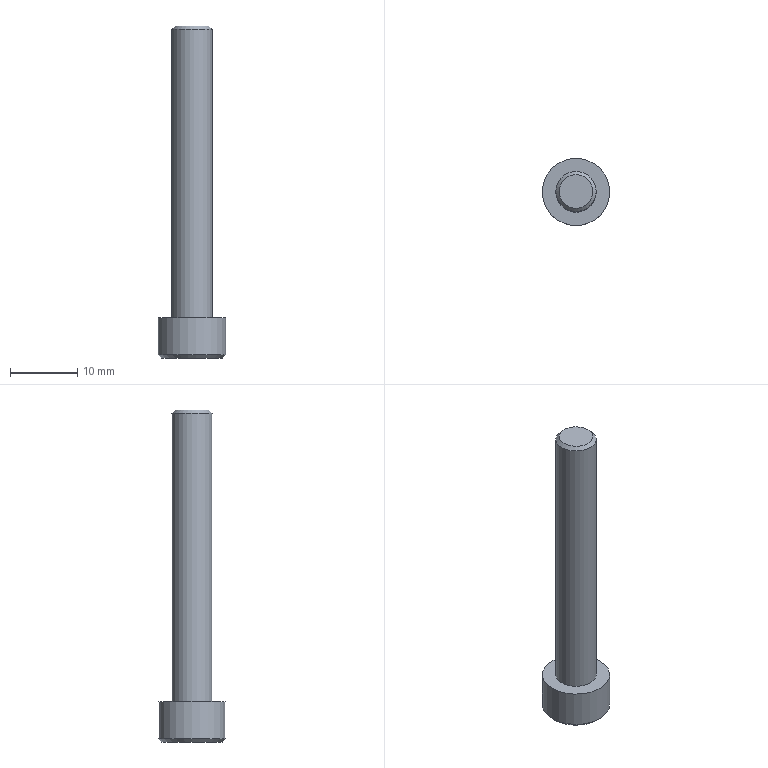Part | STEP file | M6.00-50.00 | 1 solid | 14 faces | box 10 x 10 x 49.34 mm | volume 1626 mm3 | plane 10 | cylinder 2 | cone 2 | commonest cylinder face diameters 6 x1 10 x1